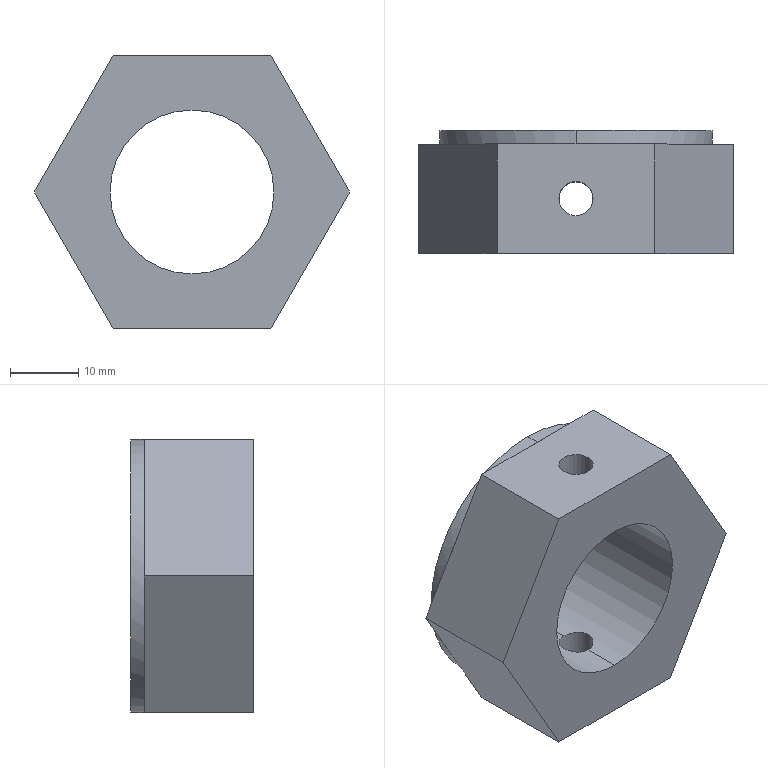Part | SolidWorks | features BaseBody 1 | 1 solid | 22 faces | box 46.188 x 18 x 40 mm | volume 16224 mm3 | plane 14 | cylinder 8 | commonest cylinder face diameters 5 x4 24 x2 40 x2
STEP:
#1=CARTESIAN_POINT('',(0.,0.,12.));
#2=VERTEX_POINT('',#1);
#3=CARTESIAN_POINT('',(0.,0.,-12.));
#4=VERTEX_POINT('',#3);
#5=CARTESIAN_POINT('',(0.,0.,0.));
#6=DIRECTION('',(0.,-1.,0.));
#7=DIRECTION('',(0.,0.,1.));
#8=AXIS2_PLACEMENT_3D('',#5,#6,#7);
#9=CIRCLE('',#8,12.);
#10=EDGE_CURVE('',#2,#4,#9,.T.);
#11=ORIENTED_EDGE('',*,*,#10,.T.);
#12=CARTESIAN_POINT('',(0.,5.5,-12.));
#13=VERTEX_POINT('',#12);
#14=CARTESIAN_POINT('',(0.,18.,-12.));
#15=DIRECTION('',(0.,1.,0.));
#16=VECTOR('',#15,1000.);
#17=LINE('',#14,#16);
#18=EDGE_CURVE('',#4,#13,#17,.T.);
#19=ORIENTED_EDGE('',*,*,#18,.T.);
#20=CARTESIAN_POINT('',(-2.5,8.,-11.737));
#21=VERTEX_POINT('',#20);
#22=CARTESIAN_POINT('',(-2.5,8.,-11.737));
#23=CARTESIAN_POINT('',(-2.5,7.834,-11.737));
#24=CARTESIAN_POINT('',(-2.484,7.672,-11.74));
#25=CARTESIAN_POINT('',(-2.42,7.352,-11.753));
#26=CARTESIAN_POINT('',(-2.372,7.193,-11.763));
#27=CARTESIAN_POINT('',(-2.246,6.89,-11.788));
#28=CARTESIAN_POINT('',(-2.17,6.747,-11.803));
#29=CARTESIAN_POINT('',(-1.988,6.476,-11.834));
#30=CARTESIAN_POINT('',(-1.883,6.348,-11.852));
#31=CARTESIAN_POINT('',(-1.539,6.003,-11.903));
#32=CARTESIAN_POINT('',(-1.261,5.817,-11.937));
#33=CARTESIAN_POINT('',(-0.6599,5.567,-11.986));
#34=CARTESIAN_POINT('',(-0.3311,5.5,-12.));
#35=CARTESIAN_POINT('',(0.,5.5,-12.));
#36=B_SPLINE_CURVE_WITH_KNOTS('',3,(#22,#23,#24,#25,#26,#27,#28,#29,#30,#31,#32,#33,#34,#35),.UNSPECIFIED.,.F.,.F.,(4,2,2,2,2,2,4),(0.,0.0004895,0.000979,0.001469,0.001958,0.002937,0.003916),.UNSPECIFIED.);
#37=EDGE_CURVE('',#21,#13,#36,.T.);
#38=ORIENTED_EDGE('',*,*,#37,.F.);
#39=CARTESIAN_POINT('',(0.,10.5,-12.));
#40=VERTEX_POINT('',#39);
#41=CARTESIAN_POINT('',(0.,10.5,-12.));
#42=CARTESIAN_POINT('',(-0.1656,10.5,-12.));
#43=CARTESIAN_POINT('',(-0.3283,10.484,-11.997));
#44=CARTESIAN_POINT('',(-0.6482,10.42,-11.984));
#45=CARTESIAN_POINT('',(-0.8072,10.372,-11.974));
#46=CARTESIAN_POINT('',(-1.11,10.246,-11.95));
#47=CARTESIAN_POINT('',(-1.253,10.17,-11.935));
#48=CARTESIAN_POINT('',(-1.524,9.988,-11.904));
#49=CARTESIAN_POINT('',(-1.652,9.883,-11.886));
#50=CARTESIAN_POINT('',(-1.997,9.539,-11.835));
#51=CARTESIAN_POINT('',(-2.183,9.261,-11.8));
#52=CARTESIAN_POINT('',(-2.433,8.66,-11.751));
#53=CARTESIAN_POINT('',(-2.5,8.331,-11.737));
#54=CARTESIAN_POINT('',(-2.5,8.,-11.737));
#55=B_SPLINE_CURVE_WITH_KNOTS('',3,(#41,#42,#43,#44,#45,#46,#47,#48,#49,#50,#51,#52,#53,#54),.UNSPECIFIED.,.F.,.F.,(4,2,2,2,2,2,4),(-0.003916,-0.003427,-0.002937,-0.002448,-0.001958,-0.000979,0.),.UNSPECIFIED.);
#56=EDGE_CURVE('',#40,#21,#55,.T.);
#57=ORIENTED_EDGE('',*,*,#56,.F.);
#58=CARTESIAN_POINT('',(0.,18.,-12.));
#59=VERTEX_POINT('',#58);
#60=CARTESIAN_POINT('',(0.,18.,-12.));
#61=DIRECTION('',(0.,1.,0.));
#62=VECTOR('',#61,1000.);
#63=LINE('',#60,#62);
#64=EDGE_CURVE('',#40,#59,#63,.T.);
#65=ORIENTED_EDGE('',*,*,#64,.T.);
#66=CARTESIAN_POINT('',(0.,18.,12.));
#67=VERTEX_POINT('',#66);
#68=CARTESIAN_POINT('',(0.,18.,0.));
#69=DIRECTION('',(0.,-1.,0.));
#70=DIRECTION('',(0.,0.,1.));
#71=AXIS2_PLACEMENT_3D('',#68,#69,#70);
#72=CIRCLE('',#71,12.);
#73=EDGE_CURVE('',#67,#59,#72,.T.);
#74=ORIENTED_EDGE('',*,*,#73,.F.);
#75=CARTESIAN_POINT('',(0.,10.5,12.));
#76=VERTEX_POINT('',#75);
#77=CARTESIAN_POINT('',(0.,18.,12.));
#78=DIRECTION('',(0.,1.,0.));
#79=VECTOR('',#78,1000.);
#80=LINE('',#77,#79);
#81=EDGE_CURVE('',#76,#67,#80,.T.);
#82=ORIENTED_EDGE('',*,*,#81,.F.);
#83=CARTESIAN_POINT('',(-2.5,8.,11.737));
#84=VERTEX_POINT('',#83);
#85=CARTESIAN_POINT('',(-2.5,8.,11.737));
#86=CARTESIAN_POINT('',(-2.5,8.166,11.737));
#87=CARTESIAN_POINT('',(-2.484,8.328,11.74));
#88=CARTESIAN_POINT('',(-2.42,8.648,11.753));
#89=CARTESIAN_POINT('',(-2.372,8.807,11.763));
#90=CARTESIAN_POINT('',(-2.246,9.11,11.788));
#91=CARTESIAN_POINT('',(-2.17,9.253,11.803));
#92=CARTESIAN_POINT('',(-1.988,9.524,11.834));
#93=CARTESIAN_POINT('',(-1.883,9.652,11.852));
#94=CARTESIAN_POINT('',(-1.539,9.997,11.903));
#95=CARTESIAN_POINT('',(-1.261,10.183,11.937));
#96=CARTESIAN_POINT('',(-0.6599,10.433,11.986));
#97=CARTESIAN_POINT('',(-0.3311,10.5,12.));
#98=CARTESIAN_POINT('',(0.,10.5,12.));
#99=B_SPLINE_CURVE_WITH_KNOTS('',3,(#85,#86,#87,#88,#89,#90,#91,#92,#93,#94,#95,#96,#97,#98),.UNSPECIFIED.,.F.,.F.,(4,2,2,2,2,2,4),(0.,0.0004895,0.000979,0.001469,0.001958,0.002937,0.003916),.UNSPECIFIED.);
#100=EDGE_CURVE('',#84,#76,#99,.T.);
#101=ORIENTED_EDGE('',*,*,#100,.F.);
#102=CARTESIAN_POINT('',(0.,5.5,12.));
#103=VERTEX_POINT('',#102);
#104=CARTESIAN_POINT('',(0.,5.5,12.));
#105=CARTESIAN_POINT('',(-0.1656,5.5,12.));
#106=CARTESIAN_POINT('',(-0.3283,5.516,11.997));
#107=CARTESIAN_POINT('',(-0.6482,5.58,11.984));
#108=CARTESIAN_POINT('',(-0.8072,5.628,11.974));
#109=CARTESIAN_POINT('',(-1.11,5.754,11.95));
#110=CARTESIAN_POINT('',(-1.253,5.83,11.935));
#111=CARTESIAN_POINT('',(-1.524,6.012,11.904));
#112=CARTESIAN_POINT('',(-1.652,6.117,11.886));
#113=CARTESIAN_POINT('',(-1.997,6.461,11.835));
#114=CARTESIAN_POINT('',(-2.183,6.739,11.8));
#115=CARTESIAN_POINT('',(-2.433,7.34,11.751));
#116=CARTESIAN_POINT('',(-2.5,7.669,11.737));
#117=CARTESIAN_POINT('',(-2.5,8.,11.737));
#118=B_SPLINE_CURVE_WITH_KNOTS('',3,(#104,#105,#106,#107,#108,#109,#110,#111,#112,#113,#114,#115,#116,#117),.UNSPECIFIED.,.F.,.F.,(4,2,2,2,2,2,4),(-0.003916,-0.003427,-0.002937,-0.002448,-0.001958,-0.000979,0.),.UNSPECIFIED.);
#119=EDGE_CURVE('',#103,#84,#118,.T.);
#120=ORIENTED_EDGE('',*,*,#119,.F.);
#121=CARTESIAN_POINT('',(0.,18.,12.));
#122=DIRECTION('',(0.,1.,0.));
#123=VECTOR('',#122,1000.);
#124=LINE('',#121,#123);
#125=EDGE_CURVE('',#2,#103,#124,.T.);
#126=ORIENTED_EDGE('',*,*,#125,.F.);
#127=EDGE_LOOP('',(#11,#19,#38,#57,#65,#74,#82,#101,#120,#126));
#128=FACE_OUTER_BOUND('',#127,.T.);
#129=CARTESIAN_POINT('',(0.,18.,0.));
#130=DIRECTION('',(0.,1.,0.));
#131=DIRECTION('',(0.,0.,1.));
#132=AXIS2_PLACEMENT_3D('',#129,#130,#131);
#133=CYLINDRICAL_SURFACE('',#132,12.);
#134=ADVANCED_FACE('',(#128),#133,.F.);
#135=CARTESIAN_POINT('',(2.5,8.,-20.));
#136=VERTEX_POINT('',#135);
#137=CARTESIAN_POINT('',(-2.5,8.,-20.));
#138=VERTEX_POINT('',#137);
#139=CARTESIAN_POINT('',(0.,8.,-20.));
#140=DIRECTION('',(0.,0.,-1.));
#141=DIRECTION('',(1.,0.,0.));
#142=AXIS2_PLACEMENT_3D('',#139,#140,#141);
#143=CIRCLE('',#142,2.5);
#144=EDGE_CURVE('',#136,#138,#143,.T.);
#145=ORIENTED_EDGE('',*,*,#144,.T.);
#146=CARTESIAN_POINT('',(-2.5,8.,20.));
#147=DIRECTION('',(0.,0.,1.));
#148=VECTOR('',#147,1000.);
#149=LINE('',#146,#148);
#150=EDGE_CURVE('',#138,#21,#149,.T.);
#151=ORIENTED_EDGE('',*,*,#150,.T.);
#152=ORIENTED_EDGE('',*,*,#37,.T.);
#153=CARTESIAN_POINT('',(2.5,8.,-11.737));
#154=VERTEX_POINT('',#153);
#155=CARTESIAN_POINT('',(0.,5.5,-12.));
#156=CARTESIAN_POINT('',(0.1656,5.5,-12.));
#157=CARTESIAN_POINT('',(0.3283,5.516,-11.997));
#158=CARTESIAN_POINT('',(0.6482,5.58,-11.984));
#159=CARTESIAN_POINT('',(0.8072,5.628,-11.974));
#160=CARTESIAN_POINT('',(1.11,5.754,-11.95));
#161=CARTESIAN_POINT('',(1.253,5.83,-11.935));
#162=CARTESIAN_POINT('',(1.524,6.012,-11.904));
#163=CARTESIAN_POINT('',(1.652,6.117,-11.886));
#164=CARTESIAN_POINT('',(1.997,6.461,-11.835));
#165=CARTESIAN_POINT('',(2.183,6.739,-11.8));
#166=CARTESIAN_POINT('',(2.433,7.34,-11.751));
#167=CARTESIAN_POINT('',(2.5,7.669,-11.737));
#168=CARTESIAN_POINT('',(2.5,8.,-11.737));
#169=B_SPLINE_CURVE_WITH_KNOTS('',3,(#155,#156,#157,#158,#159,#160,#161,#162,#163,#164,#165,#166,#167,#168),.UNSPECIFIED.,.F.,.F.,(4,2,2,2,2,2,4),(0.003916,0.004406,0.004895,0.005385,0.005874,0.006853,0.007832),.UNSPECIFIED.);
#170=EDGE_CURVE('',#13,#154,#169,.T.);
#171=ORIENTED_EDGE('',*,*,#170,.T.);
#172=CARTESIAN_POINT('',(2.5,8.,20.));
#173=DIRECTION('',(0.,0.,1.));
#174=VECTOR('',#173,1000.);
#175=LINE('',#172,#174);
#176=EDGE_CURVE('',#136,#154,#175,.T.);
#177=ORIENTED_EDGE('',*,*,#176,.F.);
#178=EDGE_LOOP('',(#145,#151,#152,#171,#177));
#179=FACE_OUTER_BOUND('',#178,.T.);
#180=CARTESIAN_POINT('',(0.,8.,20.));
#181=DIRECTION('',(0.,0.,1.));
#182=DIRECTION('',(1.,0.,0.));
#183=AXIS2_PLACEMENT_3D('',#180,#181,#182);
#184=CYLINDRICAL_SURFACE('',#183,2.5);
#185=ADVANCED_FACE('',(#179),#184,.F.);
#186=CARTESIAN_POINT('',(2.5,8.,11.737));
#187=VERTEX_POINT('',#186);
#188=CARTESIAN_POINT('',(2.5,8.,11.737));
#189=CARTESIAN_POINT('',(2.5,7.834,11.737));
#190=CARTESIAN_POINT('',(2.484,7.672,11.74));
#191=CARTESIAN_POINT('',(2.42,7.352,11.753));
#192=CARTESIAN_POINT('',(2.372,7.193,11.763));
#193=CARTESIAN_POINT('',(2.246,6.89,11.788));
#194=CARTESIAN_POINT('',(2.17,6.747,11.803));
#195=CARTESIAN_POINT('',(1.988,6.476,11.834));
#196=CARTESIAN_POINT('',(1.883,6.348,11.852));
#197=CARTESIAN_POINT('',(1.539,6.003,11.903));
#198=CARTESIAN_POINT('',(1.261,5.817,11.937));
#199=CARTESIAN_POINT('',(0.6599,5.567,11.986));
#200=CARTESIAN_POINT('',(0.3311,5.5,12.));
#201=CARTESIAN_POINT('',(0.,5.5,12.));
#202=B_SPLINE_CURVE_WITH_KNOTS('',3,(#188,#189,#190,#191,#192,#193,#194,#195,#196,#197,#198,#199,#200,#201),.UNSPECIFIED.,.F.,.F.,(4,2,2,2,2,2,4),(0.007832,0.008322,0.008811,0.009301,0.009791,0.01077,0.01175),.UNSPECIFIED.);
#203=EDGE_CURVE('',#187,#103,#202,.T.);
#204=ORIENTED_EDGE('',*,*,#203,.T.);
#205=ORIENTED_EDGE('',*,*,#119,.T.);
#206=CARTESIAN_POINT('',(-2.5,8.,20.));
#207=VERTEX_POINT('',#206);
#208=CARTESIAN_POINT('',(-2.5,8.,20.));
#209=DIRECTION('',(0.,0.,1.));
#210=VECTOR('',#209,1000.);
#211=LINE('',#208,#210);
#212=EDGE_CURVE('',#84,#207,#211,.T.);
#213=ORIENTED_EDGE('',*,*,#212,.T.);
#214=CARTESIAN_POINT('',(2.5,8.,20.));
#215=VERTEX_POINT('',#214);
#216=CARTESIAN_POINT('',(0.,8.,20.));
#217=DIRECTION('',(0.,0.,1.));
#218=DIRECTION('',(1.,0.,0.));
#219=AXIS2_PLACEMENT_3D('',#216,#217,#218);
#220=CIRCLE('',#219,2.5);
#221=EDGE_CURVE('',#207,#215,#220,.T.);
#222=ORIENTED_EDGE('',*,*,#221,.T.);
#223=CARTESIAN_POINT('',(2.5,8.,20.));
#224=DIRECTION('',(0.,0.,1.));
#225=VECTOR('',#224,1000.);
#226=LINE('',#223,#225);
#227=EDGE_CURVE('',#187,#215,#226,.T.);
#228=ORIENTED_EDGE('',*,*,#227,.F.);
#229=EDGE_LOOP('',(#204,#205,#213,#222,#228));
#230=FACE_OUTER_BOUND('',#229,.T.);
#231=CARTESIAN_POINT('',(0.,8.,20.));
#232=DIRECTION('',(0.,0.,1.));
#233=DIRECTION('',(1.,0.,0.));
#234=AXIS2_PLACEMENT_3D('',#231,#232,#233);
#235=CYLINDRICAL_SURFACE('',#234,2.5);
#236=ADVANCED_FACE('',(#230),#235,.F.);
#237=CARTESIAN_POINT('',(0.,18.,20.));
#238=VERTEX_POINT('',#237);
#239=CARTESIAN_POINT('',(0.,18.,-20.));
#240=VERTEX_POINT('',#239);
#241=CARTESIAN_POINT('',(0.,18.,0.));
#242=DIRECTION('',(0.,1.,0.));
#243=DIRECTION('',(0.,0.,-1.));
#244=AXIS2_PLACEMENT_3D('',#241,#242,#243);
#245=CIRCLE('',#244,20.);
#246=EDGE_CURVE('',#238,#240,#245,.T.);
#247=ORIENTED_EDGE('',*,*,#246,.F.);
#248=CARTESIAN_POINT('',(0.,16.,20.));
#249=VERTEX_POINT('',#248);
#250=CARTESIAN_POINT('',(0.,18.,20.));
#251=DIRECTION('',(0.,-1.,0.));
#252=VECTOR('',#251,1000.);
#253=LINE('',#250,#252);
#254=EDGE_CURVE('',#238,#249,#253,.T.);
#255=ORIENTED_EDGE('',*,*,#254,.T.);
#256=CARTESIAN_POINT('',(17.321,16.,10.));
#257=VERTEX_POINT('',#256);
#258=CARTESIAN_POINT('',(0.,16.,0.));
#259=DIRECTION('',(0.,-1.,0.));
#260=DIRECTION('',(0.,0.,-1.));
#261=AXIS2_PLACEMENT_3D('',#258,#259,#260);
#262=CIRCLE('',#261,20.);
#263=EDGE_CURVE('',#257,#249,#262,.T.);
#264=ORIENTED_EDGE('',*,*,#263,.F.);
#265=CARTESIAN_POINT('',(17.321,16.,-10.));
#266=VERTEX_POINT('',#265);
#267=CARTESIAN_POINT('',(0.,16.,0.));
#268=DIRECTION('',(0.,-1.,0.));
#269=DIRECTION('',(0.,0.,-1.));
#270=AXIS2_PLACEMENT_3D('',#267,#268,#269);
#271=CIRCLE('',#270,20.);
#272=EDGE_CURVE('',#266,#257,#271,.T.);
#273=ORIENTED_EDGE('',*,*,#272,.F.);
#274=CARTESIAN_POINT('',(0.,16.,-20.));
#275=VERTEX_POINT('',#274);
#276=CARTESIAN_POINT('',(0.,16.,0.));
#277=DIRECTION('',(0.,-1.,0.));
#278=DIRECTION('',(0.,0.,-1.));
#279=AXIS2_PLACEMENT_3D('',#276,#277,#278);
#280=CIRCLE('',#279,20.);
#281=EDGE_CURVE('',#275,#266,#280,.T.);
#282=ORIENTED_EDGE('',*,*,#281,.F.);
#283=CARTESIAN_POINT('',(0.,18.,-20.));
#284=DIRECTION('',(0.,-1.,0.));
#285=VECTOR('',#284,1000.);
#286=LINE('',#283,#285);
#287=EDGE_CURVE('',#240,#275,#286,.T.);
#288=ORIENTED_EDGE('',*,*,#287,.F.);
#289=EDGE_LOOP('',(#247,#255,#264,#273,#282,#288));
#290=FACE_OUTER_BOUND('',#289,.T.);
#291=CARTESIAN_POINT('',(0.,18.,0.));
#292=DIRECTION('',(0.,-1.,0.));
#293=DIRECTION('',(0.,0.,-1.));
#294=AXIS2_PLACEMENT_3D('',#291,#292,#293);
#295=CYLINDRICAL_SURFACE('',#294,20.);
#296=ADVANCED_FACE('',(#290),#295,.T.);
#297=ORIENTED_EDGE('',*,*,#10,.F.);
#298=CARTESIAN_POINT('',(0.,0.,0.));
#299=DIRECTION('',(0.,-1.,0.));
#300=DIRECTION('',(0.,0.,1.));
#301=AXIS2_PLACEMENT_3D('',#298,#299,#300);
#302=CIRCLE('',#301,12.);
#303=EDGE_CURVE('',#4,#2,#302,.T.);
#304=ORIENTED_EDGE('',*,*,#303,.F.);
#305=EDGE_LOOP('',(#297,#304));
#306=FACE_BOUND('',#305,.T.);
#307=CARTESIAN_POINT('',(-23.094,0.,0.));
#308=VERTEX_POINT('',#307);
#309=CARTESIAN_POINT('',(-11.547,0.,20.));
#310=VERTEX_POINT('',#309);
#311=CARTESIAN_POINT('',(-23.094,0.,0.));
#312=DIRECTION('',(0.5,0.,0.866));
#313=VECTOR('',#312,1000.);
#314=LINE('',#311,#313);
#315=EDGE_CURVE('',#308,#310,#314,.T.);
#316=ORIENTED_EDGE('',*,*,#315,.F.);
#317=CARTESIAN_POINT('',(-11.547,0.,-20.));
#318=VERTEX_POINT('',#317);
#319=CARTESIAN_POINT('',(-11.547,0.,-20.));
#320=DIRECTION('',(-0.5,0.,0.866));
#321=VECTOR('',#320,1000.);
#322=LINE('',#319,#321);
#323=EDGE_CURVE('',#318,#308,#322,.T.);
#324=ORIENTED_EDGE('',*,*,#323,.F.);
#325=CARTESIAN_POINT('',(11.547,0.,-20.));
#326=VERTEX_POINT('',#325);
#327=CARTESIAN_POINT('',(0.,0.,-20.));
#328=DIRECTION('',(-1.,0.,0.));
#329=VECTOR('',#328,1000.);
#330=LINE('',#327,#329);
#331=EDGE_CURVE('',#326,#318,#330,.T.);
#332=ORIENTED_EDGE('',*,*,#331,.F.);
#333=CARTESIAN_POINT('',(23.094,0.,0.));
#334=VERTEX_POINT('',#333);
#335=CARTESIAN_POINT('',(23.094,0.,0.));
#336=DIRECTION('',(-0.5,0.,-0.866));
#337=VECTOR('',#336,1000.);
#338=LINE('',#335,#337);
#339=EDGE_CURVE('',#334,#326,#338,.T.);
#340=ORIENTED_EDGE('',*,*,#339,.F.);
#341=CARTESIAN_POINT('',(11.547,0.,20.));
#342=VERTEX_POINT('',#341);
#343=CARTESIAN_POINT('',(11.547,0.,20.));
#344=DIRECTION('',(0.5,0.,-0.866));
#345=VECTOR('',#344,1000.);
#346=LINE('',#343,#345);
#347=EDGE_CURVE('',#342,#334,#346,.T.);
#348=ORIENTED_EDGE('',*,*,#347,.F.);
#349=CARTESIAN_POINT('',(0.,0.,20.));
#350=DIRECTION('',(1.,0.,0.));
#351=VECTOR('',#350,1000.);
#352=LINE('',#349,#351);
#353=EDGE_CURVE('',#310,#342,#352,.T.);
#354=ORIENTED_EDGE('',*,*,#353,.F.);
#355=EDGE_LOOP('',(#316,#324,#332,#340,#348,#354));
#356=FACE_OUTER_BOUND('',#355,.T.);
#357=CARTESIAN_POINT('',(0.,0.,0.));
#358=DIRECTION('',(0.,1.,0.));
#359=DIRECTION('',(0.,0.,1.));
#360=AXIS2_PLACEMENT_3D('',#357,#358,#359);
#361=PLANE('',#360);
#362=ADVANCED_FACE('',(#306,#356),#361,.F.);
#363=ORIENTED_EDGE('',*,*,#18,.F.);
#364=ORIENTED_EDGE('',*,*,#303,.T.);
#365=ORIENTED_EDGE('',*,*,#125,.T.);
#366=ORIENTED_EDGE('',*,*,#203,.F.);
#367=CARTESIAN_POINT('',(0.,10.5,12.));
#368=CARTESIAN_POINT('',(0.1656,10.5,12.));
#369=CARTESIAN_POINT('',(0.3283,10.484,11.997));
#370=CARTESIAN_POINT('',(0.6482,10.42,11.984));
#371=CARTESIAN_POINT('',(0.8072,10.372,11.974));
#372=CARTESIAN_POINT('',(1.11,10.246,11.95));
#373=CARTESIAN_POINT('',(1.253,10.17,11.935));
#374=CARTESIAN_POINT('',(1.524,9.988,11.904));
#375=CARTESIAN_POINT('',(1.652,9.883,11.886));
#376=CARTESIAN_POINT('',(1.997,9.539,11.835));
#377=CARTESIAN_POINT('',(2.183,9.261,11.8));
#378=CARTESIAN_POINT('',(2.433,8.66,11.751));
#379=CARTESIAN_POINT('',(2.5,8.331,11.737));
#380=CARTESIAN_POINT('',(2.5,8.,11.737));
#381=B_SPLINE_CURVE_WITH_KNOTS('',3,(#367,#368,#369,#370,#371,#372,#373,#374,#375,#376,#377,#378,#379,#380),.UNSPECIFIED.,.F.,.F.,(4,2,2,2,2,2,4),(0.003916,0.004406,0.004895,0.005385,0.005874,0.006853,0.007832),.UNSPECIFIED.);
#382=EDGE_CURVE('',#76,#187,#381,.T.);
#383=ORIENTED_EDGE('',*,*,#382,.F.);
#384=ORIENTED_EDGE('',*,*,#81,.T.);
#385=CARTESIAN_POINT('',(0.,18.,0.));
#386=DIRECTION('',(0.,-1.,0.));
#387=DIRECTION('',(0.,0.,1.));
#388=AXIS2_PLACEMENT_3D('',#385,#386,#387);
#389=CIRCLE('',#388,12.);
#390=EDGE_CURVE('',#59,#67,#389,.T.);
#391=ORIENTED_EDGE('',*,*,#390,.F.);
#392=ORIENTED_EDGE('',*,*,#64,.F.);
#393=CARTESIAN_POINT('',(2.5,8.,-11.737));
#394=CARTESIAN_POINT('',(2.5,8.166,-11.737));
#395=CARTESIAN_POINT('',(2.484,8.328,-11.74));
#396=CARTESIAN_POINT('',(2.42,8.648,-11.753));
#397=CARTESIAN_POINT('',(2.372,8.807,-11.763));
#398=CARTESIAN_POINT('',(2.246,9.11,-11.788));
#399=CARTESIAN_POINT('',(2.17,9.253,-11.803));
#400=CARTESIAN_POINT('',(1.988,9.524,-11.834));
#401=CARTESIAN_POINT('',(1.883,9.652,-11.852));
#402=CARTESIAN_POINT('',(1.539,9.997,-11.903));
#403=CARTESIAN_POINT('',(1.261,10.183,-11.937));
#404=CARTESIAN_POINT('',(0.6599,10.433,-11.986));
#405=CARTESIAN_POINT('',(0.3311,10.5,-12.));
#406=CARTESIAN_POINT('',(0.,10.5,-12.));
#407=B_SPLINE_CURVE_WITH_KNOTS('',3,(#393,#394,#395,#396,#397,#398,#399,#400,#401,#402,#403,#404,#405,#406),.UNSPECIFIED.,.F.,.F.,(4,2,2,2,2,2,4),(0.007832,0.008322,0.008811,0.009301,0.009791,0.01077,0.01175),.UNSPECIFIED.);
#408=EDGE_CURVE('',#154,#40,#407,.T.);
#409=ORIENTED_EDGE('',*,*,#408,.F.);
#410=ORIENTED_EDGE('',*,*,#170,.F.);
#411=EDGE_LOOP('',(#363,#364,#365,#366,#383,#384,#391,#392,#409,#410));
#412=FACE_OUTER_BOUND('',#411,.T.);
#413=CARTESIAN_POINT('',(0.,18.,0.));
#414=DIRECTION('',(0.,1.,0.));
#415=DIRECTION('',(0.,0.,1.));
#416=AXIS2_PLACEMENT_3D('',#413,#414,#415);
#417=CYLINDRICAL_SURFACE('',#416,12.);
#418=ADVANCED_FACE('',(#412),#417,.F.);
#419=CARTESIAN_POINT('',(0.,8.,20.));
#420=DIRECTION('',(0.,0.,1.));
#421=DIRECTION('',(1.,0.,0.));
#422=AXIS2_PLACEMENT_3D('',#419,#420,#421);
#423=CIRCLE('',#422,2.5);
#424=EDGE_CURVE('',#215,#207,#423,.T.);
#425=ORIENTED_EDGE('',*,*,#424,.F.);
#426=ORIENTED_EDGE('',*,*,#221,.F.);
#427=EDGE_LOOP('',(#425,#426));
#428=FACE_BOUND('',#427,.T.);
#429=CARTESIAN_POINT('',(11.547,16.,20.));
#430=VERTEX_POINT('',#429);
#431=CARTESIAN_POINT('',(-11.547,16.,20.));
#432=DIRECTION('',(1.,0.,0.));
#433=VECTOR('',#432,1000.);
#434=LINE('',#431,#433);
#435=EDGE_CURVE('',#249,#430,#434,.T.);
#436=ORIENTED_EDGE('',*,*,#435,.F.);
#437=CARTESIAN_POINT('',(-11.547,16.,20.));
#438=VERTEX_POINT('',#437);
#439=CARTESIAN_POINT('',(-11.547,16.,20.));
#440=DIRECTION('',(1.,0.,0.));
#441=VECTOR('',#440,1000.);
#442=LINE('',#439,#441);
#443=EDGE_CURVE('',#438,#249,#442,.T.);
#444=ORIENTED_EDGE('',*,*,#443,.F.);
#445=CARTESIAN_POINT('',(-11.547,16.,20.));
#446=DIRECTION('',(0.,1.,0.));
#447=VECTOR('',#446,1000.);
#448=LINE('',#445,#447);
#449=EDGE_CURVE('',#310,#438,#448,.T.);
#450=ORIENTED_EDGE('',*,*,#449,.F.);
#451=ORIENTED_EDGE('',*,*,#353,.T.);
#452=CARTESIAN_POINT('',(11.547,16.,20.));
#453=DIRECTION('',(0.,-1.,0.));
#454=VECTOR('',#453,1000.);
#455=LINE('',#452,#454);
#456=EDGE_CURVE('',#430,#342,#455,.T.);
#457=ORIENTED_EDGE('',*,*,#456,.F.);
#458=EDGE_LOOP('',(#436,#444,#450,#451,#457));
#459=FACE_OUTER_BOUND('',#458,.T.);
#460=CARTESIAN_POINT('',(-11.547,16.,20.));
#461=DIRECTION('',(0.,0.,-1.));
#462=DIRECTION('',(-1.,0.,0.));
#463=AXIS2_PLACEMENT_3D('',#460,#461,#462);
#464=PLANE('',#463);
#465=ADVANCED_FACE('',(#428,#459),#464,.F.);
#466=CARTESIAN_POINT('',(-17.321,16.,10.));
#467=VERTEX_POINT('',#466);
#468=CARTESIAN_POINT('',(-23.094,16.,0.));
#469=DIRECTION('',(0.5,0.,0.866));
#470=VECTOR('',#469,1000.);
#471=LINE('',#468,#470);
#472=EDGE_CURVE('',#467,#438,#471,.T.);
#473=ORIENTED_EDGE('',*,*,#472,.F.);
#474=CARTESIAN_POINT('',(-23.094,16.,0.));
#475=VERTEX_POINT('',#474);
#476=CARTESIAN_POINT('',(-23.094,16.,0.));
#477=DIRECTION('',(0.5,0.,0.866));
#478=VECTOR('',#477,1000.);
#479=LINE('',#476,#478);
#480=EDGE_CURVE('',#475,#467,#479,.T.);
#481=ORIENTED_EDGE('',*,*,#480,.F.);
#482=CARTESIAN_POINT('',(-23.094,16.,0.));
#483=DIRECTION('',(0.,1.,0.));
#484=VECTOR('',#483,1000.);
#485=LINE('',#482,#484);
#486=EDGE_CURVE('',#308,#475,#485,.T.);
#487=ORIENTED_EDGE('',*,*,#486,.F.);
#488=ORIENTED_EDGE('',*,*,#315,.T.);
#489=ORIENTED_EDGE('',*,*,#449,.T.);
#490=EDGE_LOOP('',(#473,#481,#487,#488,#489));
#491=FACE_OUTER_BOUND('',#490,.T.);
#492=CARTESIAN_POINT('',(-23.094,16.,0.));
#493=DIRECTION('',(0.866,0.,-0.5));
#494=DIRECTION('',(-0.5,0.,-0.866));
#495=AXIS2_PLACEMENT_3D('',#492,#493,#494);
#496=PLANE('',#495);
#497=ADVANCED_FACE('',(#491),#496,.F.);
#498=CARTESIAN_POINT('',(-17.321,16.,-10.));
#499=VERTEX_POINT('',#498);
#500=CARTESIAN_POINT('',(-11.547,16.,-20.));
#501=DIRECTION('',(-0.5,0.,0.866));
#502=VECTOR('',#501,1000.);
#503=LINE('',#500,#502);
#504=EDGE_CURVE('',#499,#475,#503,.T.);
#505=ORIENTED_EDGE('',*,*,#504,.F.);
#506=CARTESIAN_POINT('',(-11.547,16.,-20.));
#507=VERTEX_POINT('',#506);
#508=CARTESIAN_POINT('',(-11.547,16.,-20.));
#509=DIRECTION('',(-0.5,0.,0.866));
#510=VECTOR('',#509,1000.);
#511=LINE('',#508,#510);
#512=EDGE_CURVE('',#507,#499,#511,.T.);
#513=ORIENTED_EDGE('',*,*,#512,.F.);
#514=CARTESIAN_POINT('',(-11.547,16.,-20.));
#515=DIRECTION('',(0.,1.,0.));
#516=VECTOR('',#515,1000.);
#517=LINE('',#514,#516);
#518=EDGE_CURVE('',#318,#507,#517,.T.);
#519=ORIENTED_EDGE('',*,*,#518,.F.);
#520=ORIENTED_EDGE('',*,*,#323,.T.);
#521=ORIENTED_EDGE('',*,*,#486,.T.);
#522=EDGE_LOOP('',(#505,#513,#519,#520,#521));
#523=FACE_OUTER_BOUND('',#522,.T.);
#524=CARTESIAN_POINT('',(-11.547,16.,-20.));
#525=DIRECTION('',(0.866,0.,0.5));
#526=DIRECTION('',(0.5,0.,-0.866));
#527=AXIS2_PLACEMENT_3D('',#524,#525,#526);
#528=PLANE('',#527);
#529=ADVANCED_FACE('',(#523),#528,.F.);
#530=ORIENTED_EDGE('',*,*,#144,.F.);
#531=CARTESIAN_POINT('',(0.,8.,-20.));
#532=DIRECTION('',(0.,0.,-1.));
#533=DIRECTION('',(1.,0.,0.));
#534=AXIS2_PLACEMENT_3D('',#531,#532,#533);
#535=CIRCLE('',#534,2.5);
#536=EDGE_CURVE('',#138,#136,#535,.T.);
#537=ORIENTED_EDGE('',*,*,#536,.F.);
#538=EDGE_LOOP('',(#530,#537));
#539=FACE_BOUND('',#538,.T.);
#540=CARTESIAN_POINT('',(11.547,16.,-20.));
#541=DIRECTION('',(-1.,0.,0.));
#542=VECTOR('',#541,1000.);
#543=LINE('',#540,#542);
#544=EDGE_CURVE('',#275,#507,#543,.T.);
#545=ORIENTED_EDGE('',*,*,#544,.F.);
#546=CARTESIAN_POINT('',(11.547,16.,-20.));
#547=VERTEX_POINT('',#546);
#548=CARTESIAN_POINT('',(11.547,16.,-20.));
#549=DIRECTION('',(-1.,0.,0.));
#550=VECTOR('',#549,1000.);
#551=LINE('',#548,#550);
#552=EDGE_CURVE('',#547,#275,#551,.T.);
#553=ORIENTED_EDGE('',*,*,#552,.F.);
#554=CARTESIAN_POINT('',(11.547,16.,-20.));
#555=DIRECTION('',(0.,1.,0.));
#556=VECTOR('',#555,1000.);
#557=LINE('',#554,#556);
#558=EDGE_CURVE('',#326,#547,#557,.T.);
#559=ORIENTED_EDGE('',*,*,#558,.F.);
#560=ORIENTED_EDGE('',*,*,#331,.T.);
#561=ORIENTED_EDGE('',*,*,#518,.T.);
#562=EDGE_LOOP('',(#545,#553,#559,#560,#561));
#563=FACE_OUTER_BOUND('',#562,.T.);
#564=CARTESIAN_POINT('',(11.547,16.,-20.));
#565=DIRECTION('',(0.,0.,1.));
#566=DIRECTION('',(1.,0.,0.));
#567=AXIS2_PLACEMENT_3D('',#564,#565,#566);
#568=PLANE('',#567);
#569=ADVANCED_FACE('',(#539,#563),#568,.F.);
#570=CARTESIAN_POINT('',(23.094,16.,0.));
#571=DIRECTION('',(-0.5,0.,-0.866));
#572=VECTOR('',#571,1000.);
#573=LINE('',#570,#572);
#574=EDGE_CURVE('',#266,#547,#573,.T.);
#575=ORIENTED_EDGE('',*,*,#574,.F.);
#576=CARTESIAN_POINT('',(23.094,16.,0.));
#577=VERTEX_POINT('',#576);
#578=CARTESIAN_POINT('',(23.094,16.,0.));
#579=DIRECTION('',(-0.5,0.,-0.866));
#580=VECTOR('',#579,1000.);
#581=LINE('',#578,#580);
#582=EDGE_CURVE('',#577,#266,#581,.T.);
#583=ORIENTED_EDGE('',*,*,#582,.F.);
#584=CARTESIAN_POINT('',(23.094,16.,0.));
#585=DIRECTION('',(0.,1.,0.));
#586=VECTOR('',#585,1000.);
#587=LINE('',#584,#586);
#588=EDGE_CURVE('',#334,#577,#587,.T.);
#589=ORIENTED_EDGE('',*,*,#588,.F.);
#590=ORIENTED_EDGE('',*,*,#339,.T.);
#591=ORIENTED_EDGE('',*,*,#558,.T.);
#592=EDGE_LOOP('',(#575,#583,#589,#590,#591));
#593=FACE_OUTER_BOUND('',#592,.T.);
#594=CARTESIAN_POINT('',(23.094,16.,0.));
#595=DIRECTION('',(-0.866,0.,0.5));
#596=DIRECTION('',(0.5,0.,0.866));
#597=AXIS2_PLACEMENT_3D('',#594,#595,#596);
#598=PLANE('',#597);
#599=ADVANCED_FACE('',(#593),#598,.F.);
#600=CARTESIAN_POINT('',(11.547,16.,20.));
#601=DIRECTION('',(0.5,0.,-0.866));
#602=VECTOR('',#601,1000.);
#603=LINE('',#600,#602);
#604=EDGE_CURVE('',#257,#577,#603,.T.);
#605=ORIENTED_EDGE('',*,*,#604,.F.);
#606=CARTESIAN_POINT('',(11.547,16.,20.));
#607=DIRECTION('',(0.5,0.,-0.866));
#608=VECTOR('',#607,1000.);
#609=LINE('',#606,#608);
#610=EDGE_CURVE('',#430,#257,#609,.T.);
#611=ORIENTED_EDGE('',*,*,#610,.F.);
#612=ORIENTED_EDGE('',*,*,#456,.T.);
#613=ORIENTED_EDGE('',*,*,#347,.T.);
#614=ORIENTED_EDGE('',*,*,#588,.T.);
#615=EDGE_LOOP('',(#605,#611,#612,#613,#614));
#616=FACE_OUTER_BOUND('',#615,.T.);
#617=CARTESIAN_POINT('',(11.547,16.,20.));
#618=DIRECTION('',(-0.866,0.,-0.5));
#619=DIRECTION('',(-0.5,0.,0.866));
#620=AXIS2_PLACEMENT_3D('',#617,#618,#619);
#621=PLANE('',#620);
#622=ADVANCED_FACE('',(#616),#621,.F.);
#623=ORIENTED_EDGE('',*,*,#150,.F.);
#624=ORIENTED_EDGE('',*,*,#536,.T.);
#625=ORIENTED_EDGE('',*,*,#176,.T.);
#626=ORIENTED_EDGE('',*,*,#408,.T.);
#627=ORIENTED_EDGE('',*,*,#56,.T.);
#628=EDGE_LOOP('',(#623,#624,#625,#626,#627));
#629=FACE_OUTER_BOUND('',#628,.T.);
#630=CARTESIAN_POINT('',(0.,8.,20.));
#631=DIRECTION('',(0.,0.,1.));
#632=DIRECTION('',(1.,0.,0.));
#633=AXIS2_PLACEMENT_3D('',#630,#631,#632);
#634=CYLINDRICAL_SURFACE('',#633,2.5);
#635=ADVANCED_FACE('',(#629),#634,.F.);
#636=ORIENTED_EDGE('',*,*,#73,.T.);
#637=ORIENTED_EDGE('',*,*,#390,.T.);
#638=EDGE_LOOP('',(#636,#637));
#639=FACE_BOUND('',#638,.T.);
#640=CARTESIAN_POINT('',(0.,18.,0.));
#641=DIRECTION('',(0.,1.,0.));
#642=DIRECTION('',(0.,0.,-1.));
#643=AXIS2_PLACEMENT_3D('',#640,#641,#642);
#644=CIRCLE('',#643,20.);
#645=EDGE_CURVE('',#240,#238,#644,.T.);
#646=ORIENTED_EDGE('',*,*,#645,.T.);
#647=ORIENTED_EDGE('',*,*,#246,.T.);
#648=EDGE_LOOP('',(#646,#647));
#649=FACE_OUTER_BOUND('',#648,.T.);
#650=CARTESIAN_POINT('',(0.,18.,0.));
#651=DIRECTION('',(0.,1.,0.));
#652=DIRECTION('',(0.,0.,1.));
#653=AXIS2_PLACEMENT_3D('',#650,#651,#652);
#654=PLANE('',#653);
#655=ADVANCED_FACE('',(#639,#649),#654,.T.);
#656=ORIENTED_EDGE('',*,*,#212,.F.);
#657=ORIENTED_EDGE('',*,*,#100,.T.);
#658=ORIENTED_EDGE('',*,*,#382,.T.);
#659=ORIENTED_EDGE('',*,*,#227,.T.);
#660=ORIENTED_EDGE('',*,*,#424,.T.);
#661=EDGE_LOOP('',(#656,#657,#658,#659,#660));
#662=FACE_OUTER_BOUND('',#661,.T.);
#663=CARTESIAN_POINT('',(0.,8.,20.));
#664=DIRECTION('',(0.,0.,1.));
#665=DIRECTION('',(1.,0.,0.));
#666=AXIS2_PLACEMENT_3D('',#663,#664,#665);
#667=CYLINDRICAL_SURFACE('',#666,2.5);
#668=ADVANCED_FACE('',(#662),#667,.F.);
#669=ORIENTED_EDGE('',*,*,#610,.T.);
#670=ORIENTED_EDGE('',*,*,#263,.T.);
#671=ORIENTED_EDGE('',*,*,#435,.T.);
#672=EDGE_LOOP('',(#669,#670,#671));
#673=FACE_OUTER_BOUND('',#672,.T.);
#674=CARTESIAN_POINT('',(0.,16.,0.));
#675=DIRECTION('',(0.,1.,0.));
#676=DIRECTION('',(0.,0.,1.));
#677=AXIS2_PLACEMENT_3D('',#674,#675,#676);
#678=PLANE('',#677);
#679=ADVANCED_FACE('',(#673),#678,.T.);
#680=ORIENTED_EDGE('',*,*,#443,.T.);
#681=CARTESIAN_POINT('',(0.,16.,0.));
#682=DIRECTION('',(0.,-1.,0.));
#683=DIRECTION('',(0.,0.,-1.));
#684=AXIS2_PLACEMENT_3D('',#681,#682,#683);
#685=CIRCLE('',#684,20.);
#686=EDGE_CURVE('',#249,#467,#685,.T.);
#687=ORIENTED_EDGE('',*,*,#686,.T.);
#688=ORIENTED_EDGE('',*,*,#472,.T.);
#689=EDGE_LOOP('',(#680,#687,#688));
#690=FACE_OUTER_BOUND('',#689,.T.);
#691=CARTESIAN_POINT('',(0.,16.,0.));
#692=DIRECTION('',(0.,1.,0.));
#693=DIRECTION('',(0.,0.,1.));
#694=AXIS2_PLACEMENT_3D('',#691,#692,#693);
#695=PLANE('',#694);
#696=ADVANCED_FACE('',(#690),#695,.T.);
#697=ORIENTED_EDGE('',*,*,#480,.T.);
#698=CARTESIAN_POINT('',(0.,16.,0.));
#699=DIRECTION('',(0.,-1.,0.));
#700=DIRECTION('',(0.,0.,-1.));
#701=AXIS2_PLACEMENT_3D('',#698,#699,#700);
#702=CIRCLE('',#701,20.);
#703=EDGE_CURVE('',#467,#499,#702,.T.);
#704=ORIENTED_EDGE('',*,*,#703,.T.);
#705=ORIENTED_EDGE('',*,*,#504,.T.);
#706=EDGE_LOOP('',(#697,#704,#705));
#707=FACE_OUTER_BOUND('',#706,.T.);
#708=CARTESIAN_POINT('',(0.,16.,0.));
#709=DIRECTION('',(0.,1.,0.));
#710=DIRECTION('',(0.,0.,1.));
#711=AXIS2_PLACEMENT_3D('',#708,#709,#710);
#712=PLANE('',#711);
#713=ADVANCED_FACE('',(#707),#712,.T.);
#714=ORIENTED_EDGE('',*,*,#512,.T.);
#715=CARTESIAN_POINT('',(0.,16.,0.));
#716=DIRECTION('',(0.,-1.,0.));
#717=DIRECTION('',(0.,0.,-1.));
#718=AXIS2_PLACEMENT_3D('',#715,#716,#717);
#719=CIRCLE('',#718,20.);
#720=EDGE_CURVE('',#499,#275,#719,.T.);
#721=ORIENTED_EDGE('',*,*,#720,.T.);
#722=ORIENTED_EDGE('',*,*,#544,.T.);
#723=EDGE_LOOP('',(#714,#721,#722));
#724=FACE_OUTER_BOUND('',#723,.T.);
#725=CARTESIAN_POINT('',(0.,16.,0.));
#726=DIRECTION('',(0.,1.,0.));
#727=DIRECTION('',(0.,0.,1.));
#728=AXIS2_PLACEMENT_3D('',#725,#726,#727);
#729=PLANE('',#728);
#730=ADVANCED_FACE('',(#724),#729,.T.);
#731=ORIENTED_EDGE('',*,*,#552,.T.);
#732=ORIENTED_EDGE('',*,*,#281,.T.);
#733=ORIENTED_EDGE('',*,*,#574,.T.);
#734=EDGE_LOOP('',(#731,#732,#733));
#735=FACE_OUTER_BOUND('',#734,.T.);
#736=CARTESIAN_POINT('',(0.,16.,0.));
#737=DIRECTION('',(0.,1.,0.));
#738=DIRECTION('',(0.,0.,1.));
#739=AXIS2_PLACEMENT_3D('',#736,#737,#738);
#740=PLANE('',#739);
#741=ADVANCED_FACE('',(#735),#740,.T.);
#742=ORIENTED_EDGE('',*,*,#582,.T.);
#743=ORIENTED_EDGE('',*,*,#272,.T.);
#744=ORIENTED_EDGE('',*,*,#604,.T.);
#745=EDGE_LOOP('',(#742,#743,#744));
#746=FACE_OUTER_BOUND('',#745,.T.);
#747=CARTESIAN_POINT('',(0.,16.,0.));
#748=DIRECTION('',(0.,1.,0.));
#749=DIRECTION('',(0.,0.,1.));
#750=AXIS2_PLACEMENT_3D('',#747,#748,#749);
#751=PLANE('',#750);
#752=ADVANCED_FACE('',(#746),#751,.T.);
#753=ORIENTED_EDGE('',*,*,#254,.F.);
#754=ORIENTED_EDGE('',*,*,#645,.F.);
#755=ORIENTED_EDGE('',*,*,#287,.T.);
#756=ORIENTED_EDGE('',*,*,#720,.F.);
#757=ORIENTED_EDGE('',*,*,#703,.F.);
#758=ORIENTED_EDGE('',*,*,#686,.F.);
#759=EDGE_LOOP('',(#753,#754,#755,#756,#757,#758));
#760=FACE_OUTER_BOUND('',#759,.T.);
#761=CARTESIAN_POINT('',(0.,18.,0.));
#762=DIRECTION('',(0.,-1.,0.));
#763=DIRECTION('',(0.,0.,-1.));
#764=AXIS2_PLACEMENT_3D('',#761,#762,#763);
#765=CYLINDRICAL_SURFACE('',#764,20.);
#766=ADVANCED_FACE('',(#760),#765,.T.);
#767=CLOSED_SHELL('',(#134,#185,#236,#296,#362,#418,#465,#497,#529,#569,#599,#622,#635,#655,#668,#679,#696,#713,#730,#741,#752,#766));
#768=MANIFOLD_SOLID_BREP('',#767);
#769=CARTESIAN_POINT('',(0.,0.,0.));
#770=DIRECTION('',(0.,0.,1.));
#771=DIRECTION('',(1.,0.,0.));
#772=AXIS2_PLACEMENT_3D('',#769,#770,#771);
#773=(LENGTH_UNIT()NAMED_UNIT(*)SI_UNIT(.MILLI.,.METRE.));
#774=UNCERTAINTY_MEASURE_WITH_UNIT(LENGTH_MEASURE(0.00001),#773,'','');
#775=(NAMED_UNIT(*)PLANE_ANGLE_UNIT()SI_UNIT($,.RADIAN.));
#776=(NAMED_UNIT(*)SI_UNIT($,.STERADIAN.)SOLID_ANGLE_UNIT());
#777=(GEOMETRIC_REPRESENTATION_CONTEXT(3)GLOBAL_UNCERTAINTY_ASSIGNED_CONTEXT((#774))GLOBAL_UNIT_ASSIGNED_CONTEXT((#773,#775,#776))REPRESENTATION_CONTEXT('',''));
#778=ADVANCED_BREP_SHAPE_REPRESENTATION('',(#768,#772),#777);